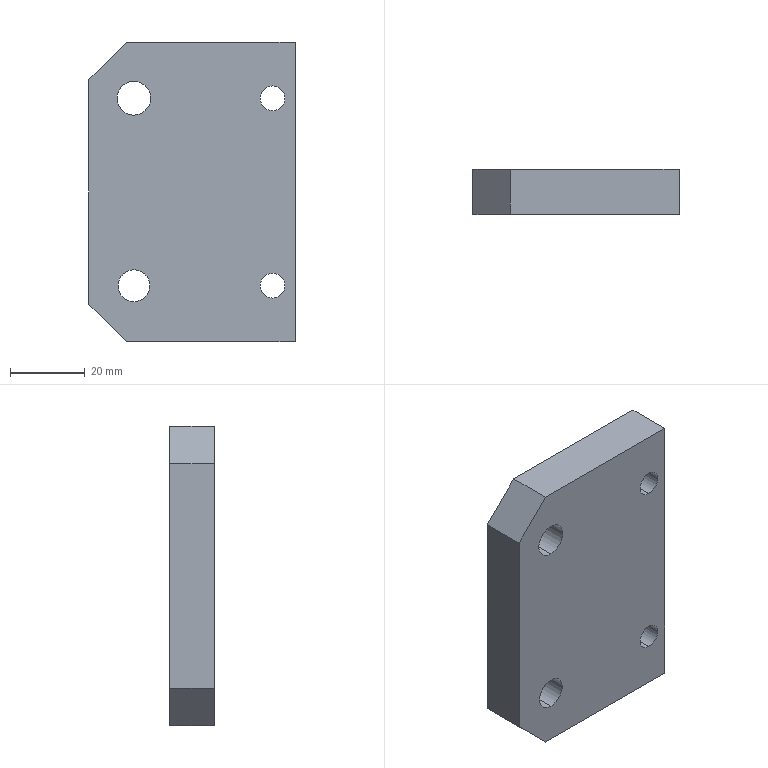Part | STEP file | PN_0047 | 1 solid | 22 faces | box 55 x 12 x 80 mm | volume 48507 mm3 | cylinder 12 | plane 10 | commonest cylinder face diameters 6.6 x4 11 x4 8.5 x2 9 x2